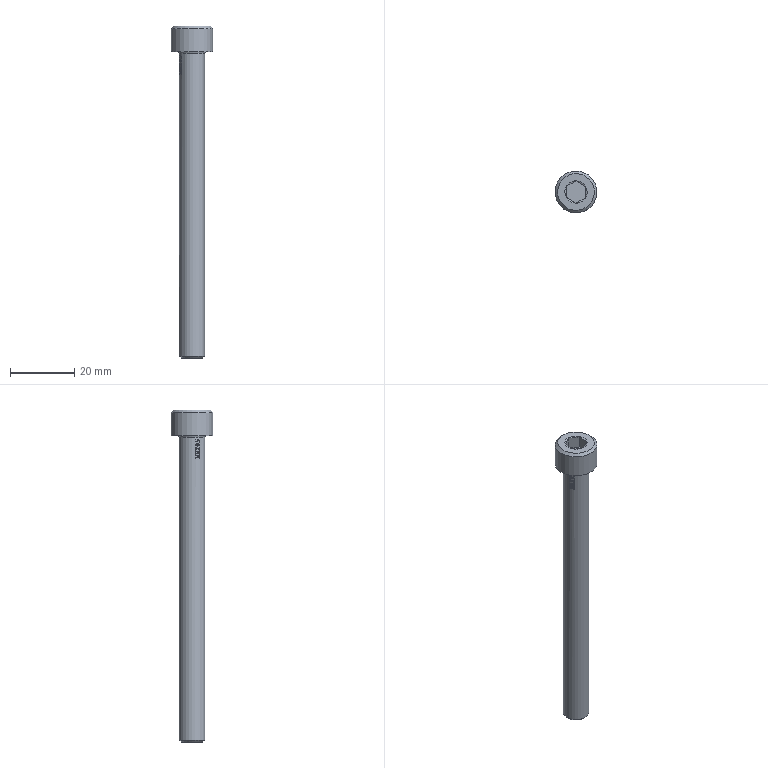Part | STEP file | solid 195 | 1 solid | 106 faces | box 13 x 13 x 103 mm | volume 5695 mm3 | plane 53 | other 36 | cylinder 8 | sphere 6 | cone 2 | torus 1 | commonest cylinder face diameters 8 x7 13 x1